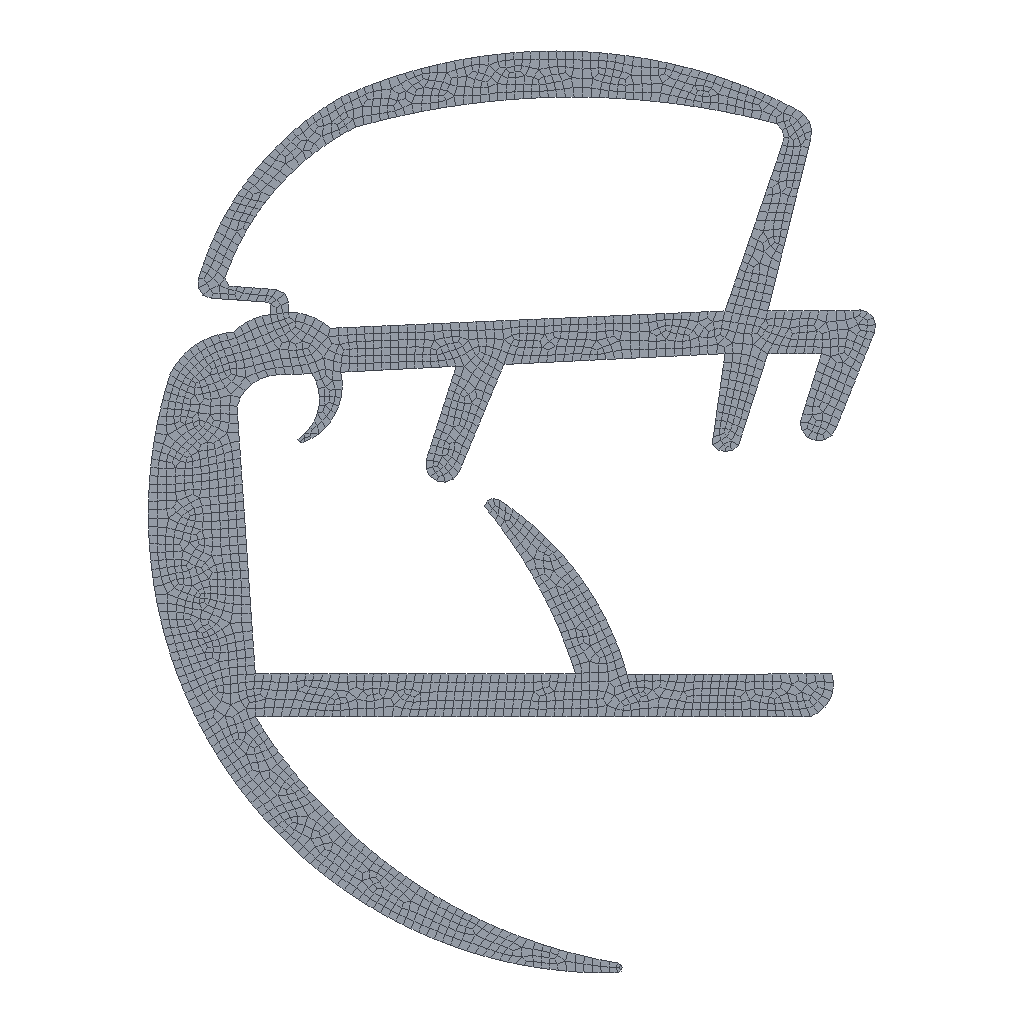Simulation study | abaqus
Set-up summary:
category,name,step,type,value,unit,region
solver,abaqus
solver,version,,,Abaqus/Standard 2020
units,not stated in the deck,,not stated
analysis,deck,,static,static
load_step,Step-1,Step-1,static
load_step,requested,,,1
mesh,nodes,,,2975
mesh,elements,,,2552
element_type,CPS4,,plane,2552
load,load commands in deck,,count,1
bc,support commands in deck,,count,4
material,MATERIAL-1,,in results
check,setup vs results,,match,"per instance, exact: element labels, types and connectivity; labels of the nodes the elements use; coordinates of those nodes at SINGLE_PRECISION in 2 of 2 instance(s)"
Abaqus input file, long lists of numbers shortened:
*Heading
** Job name: Job-1 Model name: Model-1
** Generated by: Abaqus/CAE 2020
*Preprint, echo=NO, model=NO, history=NO, contact=NO
**
** PARTS
**
*Part, name=ra
*Node
      1,   -28.36,   6.529
      2,    -27.355,   6.573
** (2972 more lines like these left out)
*Element, type=CPS4
   1,  142, 1262, 1815,  903
   2, 2351,  400, 2175, 1978
** (2550 more lines like these left out)
*Nset, nset=Set-1, generate
    1,  2974,     1
*Elset, elset=Set-1, generate
    1,  2552,     1
** Section: Section-1
*Solid Section, elset=Set-1, material=Material-1
,
*End Part
**
*Part, name=rigid
*End Part
**
**
** ASSEMBLY
**
*Assembly, name=Assembly
**
*Instance, name=ra-1, part=ra
*End Instance
**
*Instance, name=rigid-1, part=rigid
   -5.353,    23.206,           0.
*Node
      1,        -22.5,         32.5,           0.
*Nset, nset=rigid-1-RefPt_, internal
1,
*Surface, type=SEGMENTS, name=m_Surf-1
START,          -5.,           0.
 LINE,         -45.,           0.
 LINE,         -45.,         32.5
 LINE,           0.,         32.5
 LINE,           0.,           5.
 CIRCL,          -5.,           0.,       -6.875,        6.875
*Rigid Body, ref node=rigid-1-RefPt_, analytical surface=m_Surf-1
*End Instance
**
*Nset, nset=Set-1, instance=rigid-1
 1,
*Nset, nset=Set-2, instance=ra-1
   69,   70,   71,   72,   73,   74,   75,   76,   77,   78,   79,   80,   81,  147,  148,  149
  150,  151,  152,  153,  154,  155,  156,  157,  158,  159,  160,  161,  162,  163,  164,  165
** (32 more lines like these left out)
*Elset, elset=Set-2, instance=ra-1
    3,    4,    5,   24,   25,   27,   40,   43,   46,   47,   57,   66,   67,   68,   69,   70
   81,   85,   89,   90,   91,   92,   93,   94,   96,   97,   98,  100,  101,  260,  262,  263
** (31 more lines like these left out)
*Elset, elset=_s_Surf-1_S3, internal, instance=ra-1
  135,  136,  138,  143,  146,  150,  153,  159,  163,  172,  196,  197,  208,  232,  234,  238
  307,  308,  310,  311,  318,  319,  331,  332,  812,  848, 1078, 1079, 1083, 1090, 1617, 1631
** (1 more lines like these left out)
*Elset, elset=_s_Surf-1_S1, internal, instance=ra-1
  142,  149,  151,  173,  174,  175,  183,  184,  190,  207,  314,  315,  317,  322,  328,  329
  852, 1069, 1071, 1073, 1074, 1075, 1076, 1081, 1082, 1084, 1088, 1092, 1093, 1094, 1362, 1371
** (1 more lines like these left out)
*Elset, elset=_s_Surf-1_S4, internal, instance=ra-1
  205,  230, 1085, 1086, 1087, 1359, 1369, 2461
*Elset, elset=_s_Surf-1_S2, internal, instance=ra-1
  825, 1095, 1615
*Surface, type=ELEMENT, name=s_Surf-1
_s_Surf-1_S3, S3
_s_Surf-1_S1, S1
_s_Surf-1_S4, S4
_s_Surf-1_S2, S2
*End Assembly
**
** MATERIALS
**
*Material, name=Material-1
*Density
 1e-09,
*Hyperelastic, mooney-rivlin
 0.144, 0.036,    0.
**
** INTERACTION PROPERTIES
**
*Surface Interaction, name=IntProp-1
1.,
*Friction, slip tolerance=0.005
 0.2,
*Surface Behavior, pressure-overclosure=HARD
**
** INTERACTIONS
**
** Interaction: Int-1
*Contact Pair, interaction=IntProp-1, type=SURFACE TO SURFACE
s_Surf-1, rigid-1.m_Surf-1
** ----------------------------------------------------------------
**
** STEP: Step-1
**
*Step, name=Step-1, nlgeom=YES, inc=10000
*Static, stabilize=0.0002, allsdtol=0.05, continue=NO
0.001, 1., 1e-05, 1.
**
** BOUNDARY CONDITIONS
**
** Name: BC-1 Type: 位移/转角
*Boundary
Set-1, 1, 1
Set-1, 2, 2, -2.7
Set-1, 6, 6
** Name: BC-2 Type: 对称/反对称/完全固定
*Boundary
Set-2, ENCASTRE
**
** OUTPUT REQUESTS
**
*Restart, write, frequency=0
**
** FIELD OUTPUT: F-Output-1
**
*Output, field
*Node Output
CF, RF, U, V
*Element Output, directions=YES
E, LE, MISES, PE, PEEQ, PEMAG, S
*Contact Output
CDISP, CSTRESS
**
** HISTORY OUTPUT: H-Output-1
**
*Output, history, variable=PRESELECT
*End Step
Results summary:
result,step,,completed,increments=17 time=1.0/1.0
result,analysis,,,static
result,last_loadstep,,,1
result,primary field,,,U
result,reaction total,,FX,-1e-06,model units
result,reaction total,,FY,-5e-05,model units
result,reaction total,,FZ,0.0,model units